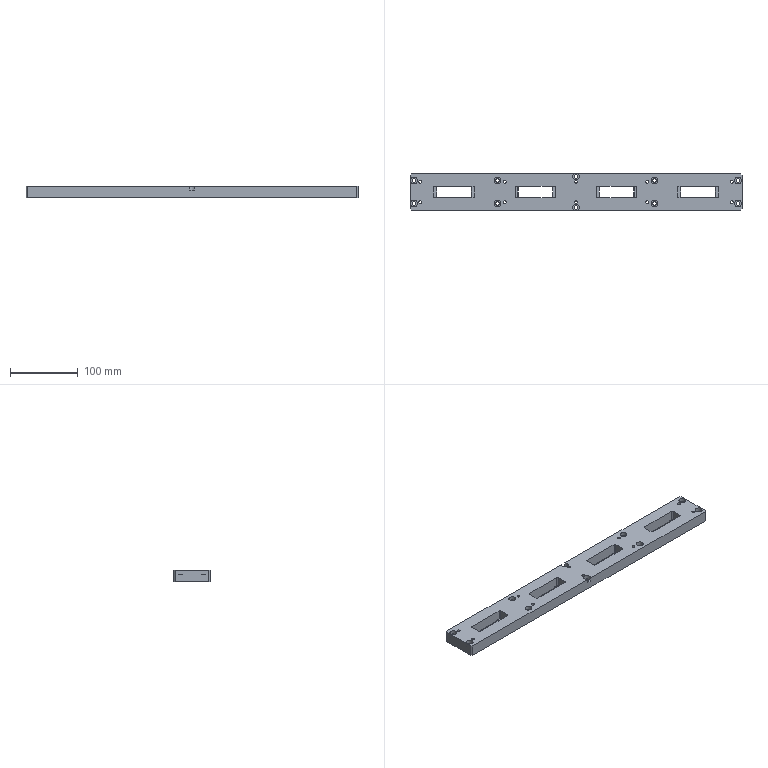Part | 1 solid | 914 faces | box 490 x 54 x 17 mm | volume 371091 mm3 | plane 473 | spline 343 | cylinder 64 | cone 34 | commonest cylinder face diameters 4 x32 4.2 x10 5.5 x10 10 x10 5 x2